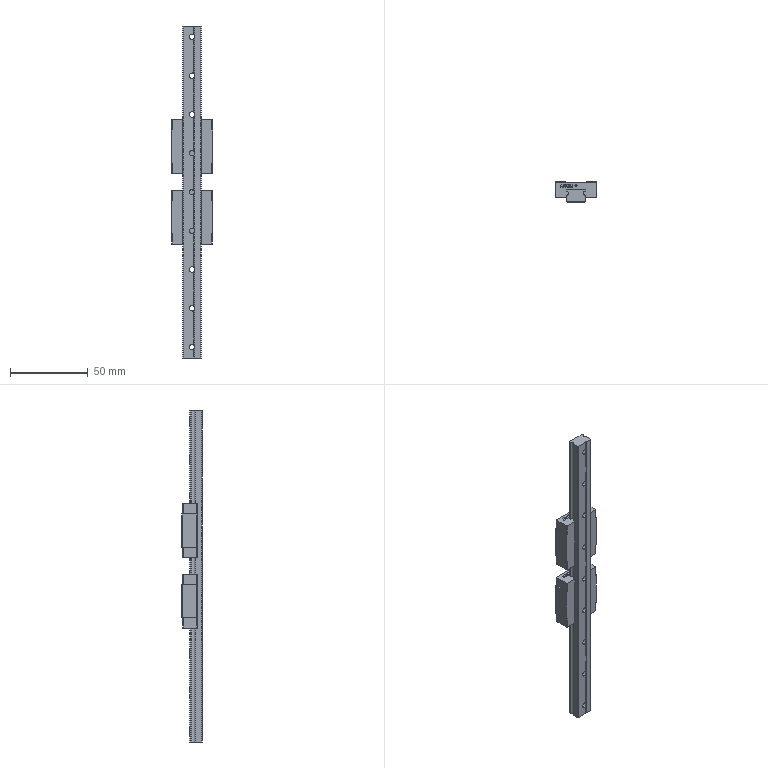Part | SolidWorks | 3 solids | 462 faces | box 27 x 13 x 214 mm | volume 32172 mm3 | plane 268 | spline 96 | cylinder 74 | cone 24 | commonest cylinder face diameters 3.5 x18 6 x18 3 x16 2.5 x9 1.4 x8 0.6 x5